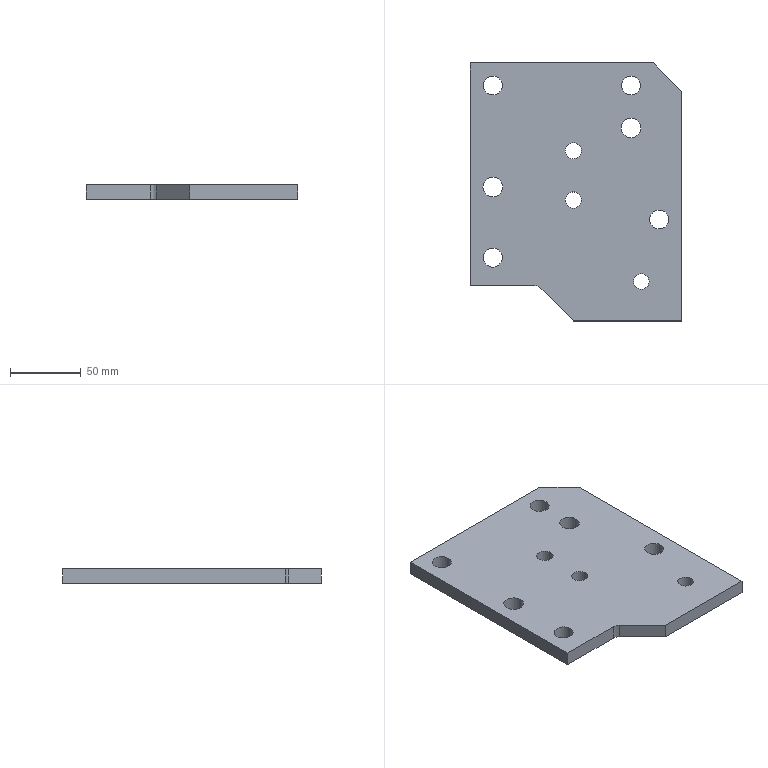Part | STEP file | lll_id126_x_t | 1 solid | 19 faces | box 150 x 183 x 10 mm | volume 245447 mm3 | cylinder 10 | plane 9 | commonest cylinder face diameters 13.509 x4 11.5 x2 14 x2 11 x1 12 x1
STEP:
#1=CARTESIAN_POINT('',(691.354,184.425,92.5));
#2=VERTEX_POINT('',#1);
#3=CARTESIAN_POINT('',(821.354,184.425,92.5));
#4=VERTEX_POINT('',#3);
#5=CARTESIAN_POINT('',(691.354,184.425,92.5));
#6=DIRECTION('',(1.,0.,0.));
#7=VECTOR('',#6,1.);
#8=LINE('',#5,#7);
#9=EDGE_CURVE('',#2,#4,#8,.T.);
#10=ORIENTED_EDGE('',*,*,#9,.T.);
#11=CARTESIAN_POINT('',(841.354,164.425,92.5));
#12=VERTEX_POINT('',#11);
#13=CARTESIAN_POINT('',(502.889,502.889,92.5));
#14=DIRECTION('',(0.7071,-0.7071,0.));
#15=VECTOR('',#14,1.);
#16=LINE('',#13,#15);
#17=EDGE_CURVE('',#4,#12,#16,.T.);
#18=ORIENTED_EDGE('',*,*,#17,.T.);
#19=CARTESIAN_POINT('',(841.354,1.425,92.5));
#20=VERTEX_POINT('',#19);
#21=CARTESIAN_POINT('',(841.354,0.,92.5));
#22=DIRECTION('',(0.,-1.,0.));
#23=VECTOR('',#22,1.);
#24=LINE('',#21,#23);
#25=EDGE_CURVE('',#12,#20,#24,.T.);
#26=ORIENTED_EDGE('',*,*,#25,.T.);
#27=CARTESIAN_POINT('',(764.739,1.425,92.5));
#28=VERTEX_POINT('',#27);
#29=CARTESIAN_POINT('',(0.,1.425,92.5));
#30=DIRECTION('',(-1.,0.,0.));
#31=VECTOR('',#30,1.);
#32=LINE('',#29,#31);
#33=EDGE_CURVE('',#20,#28,#32,.T.);
#34=ORIENTED_EDGE('',*,*,#33,.T.);
#35=CARTESIAN_POINT('',(741.497,24.668,92.5));
#36=VERTEX_POINT('',#35);
#37=CARTESIAN_POINT('',(739.739,26.425,92.5));
#38=DIRECTION('',(0.7071,-0.7071,0.));
#39=VECTOR('',#38,1.);
#40=LINE('',#37,#39);
#41=EDGE_CURVE('',#36,#28,#40,.T.);
#42=ORIENTED_EDGE('',*,*,#41,.F.);
#43=CARTESIAN_POINT('',(737.254,26.425,92.5));
#44=VERTEX_POINT('',#43);
#45=CARTESIAN_POINT('',(737.254,20.425,92.5));
#46=DIRECTION('',(0.,0.,1.));
#47=DIRECTION('',(-1.,0.,0.));
#48=AXIS2_PLACEMENT_3D('',#45,#46,#47);
#49=CIRCLE('',#48,6.);
#50=EDGE_CURVE('',#36,#44,#49,.T.);
#51=ORIENTED_EDGE('',*,*,#50,.T.);
#52=CARTESIAN_POINT('',(691.354,26.425,92.5));
#53=VERTEX_POINT('',#52);
#54=CARTESIAN_POINT('',(821.354,26.425,92.5));
#55=DIRECTION('',(-1.,0.,0.));
#56=VECTOR('',#55,1.);
#57=LINE('',#54,#56);
#58=EDGE_CURVE('',#44,#53,#57,.T.);
#59=ORIENTED_EDGE('',*,*,#58,.T.);
#60=CARTESIAN_POINT('',(691.354,26.425,92.5));
#61=DIRECTION('',(0.,1.,0.));
#62=VECTOR('',#61,1.);
#63=LINE('',#60,#62);
#64=EDGE_CURVE('',#53,#2,#63,.T.);
#65=ORIENTED_EDGE('',*,*,#64,.T.);
#66=EDGE_LOOP('',(#10,#18,#26,#34,#42,#51,#59,#65));
#67=FACE_BOUND('',#66,.T.);
#68=CARTESIAN_POINT('',(758.725,122.222,92.5));
#69=VERTEX_POINT('',#68);
#70=CARTESIAN_POINT('',(764.475,122.222,92.5));
#71=DIRECTION('',(0.,0.,-1.));
#72=DIRECTION('',(-1.,0.,0.));
#73=AXIS2_PLACEMENT_3D('',#70,#71,#72);
#74=CIRCLE('',#73,5.75);
#75=EDGE_CURVE('',#69,#69,#74,.T.);
#76=ORIENTED_EDGE('',*,*,#75,.F.);
#77=EDGE_LOOP('',(#76));
#78=FACE_BOUND('',#77,.T.);
#79=CARTESIAN_POINT('',(798.599,168.425,92.5));
#80=VERTEX_POINT('',#79);
#81=CARTESIAN_POINT('',(805.354,168.425,92.5));
#82=DIRECTION('',(0.,0.,1.));
#83=DIRECTION('',(-1.,0.,0.));
#84=AXIS2_PLACEMENT_3D('',#81,#82,#83);
#85=CIRCLE('',#84,6.755);
#86=EDGE_CURVE('',#80,#80,#85,.T.);
#87=ORIENTED_EDGE('',*,*,#86,.T.);
#88=EDGE_LOOP('',(#87));
#89=FACE_BOUND('',#88,.T.);
#90=CARTESIAN_POINT('',(700.599,168.425,92.5));
#91=VERTEX_POINT('',#90);
#92=CARTESIAN_POINT('',(707.354,168.425,92.5));
#93=DIRECTION('',(0.,0.,1.));
#94=DIRECTION('',(-1.,0.,0.));
#95=AXIS2_PLACEMENT_3D('',#92,#93,#94);
#96=CIRCLE('',#95,6.755);
#97=EDGE_CURVE('',#91,#91,#96,.T.);
#98=ORIENTED_EDGE('',*,*,#97,.T.);
#99=EDGE_LOOP('',(#98));
#100=FACE_BOUND('',#99,.T.);
#101=CARTESIAN_POINT('',(798.353,138.425,92.5));
#102=VERTEX_POINT('',#101);
#103=CARTESIAN_POINT('',(805.354,138.425,92.5));
#104=DIRECTION('',(0.,0.,1.));
#105=DIRECTION('',(-1.,0.,0.));
#106=AXIS2_PLACEMENT_3D('',#103,#104,#105);
#107=CIRCLE('',#106,7.);
#108=EDGE_CURVE('',#102,#102,#107,.T.);
#109=ORIENTED_EDGE('',*,*,#108,.T.);
#110=EDGE_LOOP('',(#109));
#111=FACE_BOUND('',#110,.T.);
#112=CARTESIAN_POINT('',(700.353,96.425,92.5));
#113=VERTEX_POINT('',#112);
#114=CARTESIAN_POINT('',(707.354,96.425,92.5));
#115=DIRECTION('',(0.,0.,1.));
#116=DIRECTION('',(-1.,0.,0.));
#117=AXIS2_PLACEMENT_3D('',#114,#115,#116);
#118=CIRCLE('',#117,7.);
#119=EDGE_CURVE('',#113,#113,#118,.T.);
#120=ORIENTED_EDGE('',*,*,#119,.T.);
#121=EDGE_LOOP('',(#120));
#122=FACE_BOUND('',#121,.T.);
#123=CARTESIAN_POINT('',(818.599,73.425,92.5));
#124=VERTEX_POINT('',#123);
#125=CARTESIAN_POINT('',(825.354,73.425,92.5));
#126=DIRECTION('',(0.,0.,1.));
#127=DIRECTION('',(-1.,0.,0.));
#128=AXIS2_PLACEMENT_3D('',#125,#126,#127);
#129=CIRCLE('',#128,6.755);
#130=EDGE_CURVE('',#124,#124,#129,.T.);
#131=ORIENTED_EDGE('',*,*,#130,.T.);
#132=EDGE_LOOP('',(#131));
#133=FACE_BOUND('',#132,.T.);
#134=CARTESIAN_POINT('',(700.599,46.425,92.5));
#135=VERTEX_POINT('',#134);
#136=CARTESIAN_POINT('',(707.354,46.425,92.5));
#137=DIRECTION('',(0.,0.,1.));
#138=DIRECTION('',(-1.,0.,0.));
#139=AXIS2_PLACEMENT_3D('',#136,#137,#138);
#140=CIRCLE('',#139,6.755);
#141=EDGE_CURVE('',#135,#135,#140,.T.);
#142=ORIENTED_EDGE('',*,*,#141,.T.);
#143=EDGE_LOOP('',(#142));
#144=FACE_BOUND('',#143,.T.);
#145=CARTESIAN_POINT('',(758.725,87.222,92.5));
#146=VERTEX_POINT('',#145);
#147=CARTESIAN_POINT('',(764.475,87.222,92.5));
#148=DIRECTION('',(0.,0.,1.));
#149=DIRECTION('',(-1.,0.,0.));
#150=AXIS2_PLACEMENT_3D('',#147,#148,#149);
#151=CIRCLE('',#150,5.75);
#152=EDGE_CURVE('',#146,#146,#151,.T.);
#153=ORIENTED_EDGE('',*,*,#152,.T.);
#154=EDGE_LOOP('',(#153));
#155=FACE_BOUND('',#154,.T.);
#156=CARTESIAN_POINT('',(807.232,29.42,92.5));
#157=VERTEX_POINT('',#156);
#158=CARTESIAN_POINT('',(812.732,29.42,92.5));
#159=DIRECTION('',(0.,0.,1.));
#160=DIRECTION('',(-1.,0.,0.));
#161=AXIS2_PLACEMENT_3D('',#158,#159,#160);
#162=CIRCLE('',#161,5.5);
#163=EDGE_CURVE('',#157,#157,#162,.T.);
#164=ORIENTED_EDGE('',*,*,#163,.T.);
#165=EDGE_LOOP('',(#164));
#166=FACE_BOUND('',#165,.T.);
#167=CARTESIAN_POINT('',(0.,0.,92.5));
#168=DIRECTION('',(0.,0.,-1.));
#169=DIRECTION('',(1.,0.,0.));
#170=AXIS2_PLACEMENT_3D('',#167,#168,#169);
#171=PLANE('',#170);
#172=ADVANCED_FACE('',(#67,#78,#89,#100,#111,#122,#133,#144,#155,#166),#171,.T.);
#173=CARTESIAN_POINT('',(807.232,29.42,102.5));
#174=VERTEX_POINT('',#173);
#175=CARTESIAN_POINT('',(812.732,29.42,102.5));
#176=DIRECTION('',(0.,0.,-1.));
#177=DIRECTION('',(-1.,0.,0.));
#178=AXIS2_PLACEMENT_3D('',#175,#176,#177);
#179=CIRCLE('',#178,5.5);
#180=EDGE_CURVE('',#174,#174,#179,.T.);
#181=ORIENTED_EDGE('',*,*,#180,.T.);
#182=EDGE_LOOP('',(#181));
#183=FACE_BOUND('',#182,.T.);
#184=CARTESIAN_POINT('',(841.354,164.425,102.5));
#185=VERTEX_POINT('',#184);
#186=CARTESIAN_POINT('',(841.354,1.425,102.5));
#187=VERTEX_POINT('',#186);
#188=CARTESIAN_POINT('',(841.354,0.,102.5));
#189=DIRECTION('',(0.,-1.,0.));
#190=VECTOR('',#189,1.);
#191=LINE('',#188,#190);
#192=EDGE_CURVE('',#185,#187,#191,.T.);
#193=ORIENTED_EDGE('',*,*,#192,.F.);
#194=CARTESIAN_POINT('',(821.354,184.425,102.5));
#195=VERTEX_POINT('',#194);
#196=CARTESIAN_POINT('',(821.354,184.425,102.5));
#197=DIRECTION('',(-0.7071,0.7071,0.));
#198=VECTOR('',#197,1.);
#199=LINE('',#196,#198);
#200=EDGE_CURVE('',#185,#195,#199,.T.);
#201=ORIENTED_EDGE('',*,*,#200,.T.);
#202=CARTESIAN_POINT('',(691.354,184.425,102.5));
#203=VERTEX_POINT('',#202);
#204=CARTESIAN_POINT('',(691.354,184.425,102.5));
#205=DIRECTION('',(1.,0.,0.));
#206=VECTOR('',#205,1.);
#207=LINE('',#204,#206);
#208=EDGE_CURVE('',#203,#195,#207,.T.);
#209=ORIENTED_EDGE('',*,*,#208,.F.);
#210=CARTESIAN_POINT('',(691.354,26.425,102.5));
#211=VERTEX_POINT('',#210);
#212=CARTESIAN_POINT('',(691.354,26.425,102.5));
#213=DIRECTION('',(0.,1.,0.));
#214=VECTOR('',#213,1.);
#215=LINE('',#212,#214);
#216=EDGE_CURVE('',#211,#203,#215,.T.);
#217=ORIENTED_EDGE('',*,*,#216,.F.);
#218=CARTESIAN_POINT('',(737.254,26.425,102.5));
#219=VERTEX_POINT('',#218);
#220=CARTESIAN_POINT('',(821.354,26.425,102.5));
#221=DIRECTION('',(-1.,0.,0.));
#222=VECTOR('',#221,1.);
#223=LINE('',#220,#222);
#224=EDGE_CURVE('',#219,#211,#223,.T.);
#225=ORIENTED_EDGE('',*,*,#224,.F.);
#226=CARTESIAN_POINT('',(741.497,24.668,102.5));
#227=VERTEX_POINT('',#226);
#228=CARTESIAN_POINT('',(737.254,20.425,102.5));
#229=DIRECTION('',(0.,0.,-1.));
#230=DIRECTION('',(-1.,0.,0.));
#231=AXIS2_PLACEMENT_3D('',#228,#229,#230);
#232=CIRCLE('',#231,6.);
#233=EDGE_CURVE('',#219,#227,#232,.T.);
#234=ORIENTED_EDGE('',*,*,#233,.T.);
#235=CARTESIAN_POINT('',(764.739,1.425,102.5));
#236=VERTEX_POINT('',#235);
#237=CARTESIAN_POINT('',(739.739,26.425,102.5));
#238=DIRECTION('',(0.7071,-0.7071,0.));
#239=VECTOR('',#238,1.);
#240=LINE('',#237,#239);
#241=EDGE_CURVE('',#227,#236,#240,.T.);
#242=ORIENTED_EDGE('',*,*,#241,.T.);
#243=CARTESIAN_POINT('',(0.,1.425,102.5));
#244=DIRECTION('',(-1.,0.,0.));
#245=VECTOR('',#244,1.);
#246=LINE('',#243,#245);
#247=EDGE_CURVE('',#187,#236,#246,.T.);
#248=ORIENTED_EDGE('',*,*,#247,.F.);
#249=EDGE_LOOP('',(#193,#201,#209,#217,#225,#234,#242,#248));
#250=FACE_BOUND('',#249,.T.);
#251=CARTESIAN_POINT('',(758.725,87.222,102.5));
#252=VERTEX_POINT('',#251);
#253=CARTESIAN_POINT('',(764.475,87.222,102.5));
#254=DIRECTION('',(0.,0.,1.));
#255=DIRECTION('',(-1.,0.,0.));
#256=AXIS2_PLACEMENT_3D('',#253,#254,#255);
#257=CIRCLE('',#256,5.75);
#258=EDGE_CURVE('',#252,#252,#257,.T.);
#259=ORIENTED_EDGE('',*,*,#258,.F.);
#260=EDGE_LOOP('',(#259));
#261=FACE_BOUND('',#260,.T.);
#262=CARTESIAN_POINT('',(700.599,46.425,102.5));
#263=VERTEX_POINT('',#262);
#264=CARTESIAN_POINT('',(707.354,46.425,102.5));
#265=DIRECTION('',(0.,0.,1.));
#266=DIRECTION('',(-1.,0.,0.));
#267=AXIS2_PLACEMENT_3D('',#264,#265,#266);
#268=CIRCLE('',#267,6.755);
#269=EDGE_CURVE('',#263,#263,#268,.T.);
#270=ORIENTED_EDGE('',*,*,#269,.F.);
#271=EDGE_LOOP('',(#270));
#272=FACE_BOUND('',#271,.T.);
#273=CARTESIAN_POINT('',(818.599,73.425,102.5));
#274=VERTEX_POINT('',#273);
#275=CARTESIAN_POINT('',(825.354,73.425,102.5));
#276=DIRECTION('',(0.,0.,1.));
#277=DIRECTION('',(-1.,0.,0.));
#278=AXIS2_PLACEMENT_3D('',#275,#276,#277);
#279=CIRCLE('',#278,6.755);
#280=EDGE_CURVE('',#274,#274,#279,.T.);
#281=ORIENTED_EDGE('',*,*,#280,.F.);
#282=EDGE_LOOP('',(#281));
#283=FACE_BOUND('',#282,.T.);
#284=CARTESIAN_POINT('',(700.353,96.425,102.5));
#285=VERTEX_POINT('',#284);
#286=CARTESIAN_POINT('',(707.354,96.425,102.5));
#287=DIRECTION('',(0.,0.,1.));
#288=DIRECTION('',(-1.,0.,0.));
#289=AXIS2_PLACEMENT_3D('',#286,#287,#288);
#290=CIRCLE('',#289,7.);
#291=EDGE_CURVE('',#285,#285,#290,.T.);
#292=ORIENTED_EDGE('',*,*,#291,.F.);
#293=EDGE_LOOP('',(#292));
#294=FACE_BOUND('',#293,.T.);
#295=CARTESIAN_POINT('',(798.353,138.425,102.5));
#296=VERTEX_POINT('',#295);
#297=CARTESIAN_POINT('',(805.354,138.425,102.5));
#298=DIRECTION('',(0.,0.,1.));
#299=DIRECTION('',(-1.,0.,0.));
#300=AXIS2_PLACEMENT_3D('',#297,#298,#299);
#301=CIRCLE('',#300,7.);
#302=EDGE_CURVE('',#296,#296,#301,.T.);
#303=ORIENTED_EDGE('',*,*,#302,.F.);
#304=EDGE_LOOP('',(#303));
#305=FACE_BOUND('',#304,.T.);
#306=CARTESIAN_POINT('',(700.599,168.425,102.5));
#307=VERTEX_POINT('',#306);
#308=CARTESIAN_POINT('',(707.354,168.425,102.5));
#309=DIRECTION('',(0.,0.,1.));
#310=DIRECTION('',(-1.,0.,0.));
#311=AXIS2_PLACEMENT_3D('',#308,#309,#310);
#312=CIRCLE('',#311,6.755);
#313=EDGE_CURVE('',#307,#307,#312,.T.);
#314=ORIENTED_EDGE('',*,*,#313,.F.);
#315=EDGE_LOOP('',(#314));
#316=FACE_BOUND('',#315,.T.);
#317=CARTESIAN_POINT('',(798.599,168.425,102.5));
#318=VERTEX_POINT('',#317);
#319=CARTESIAN_POINT('',(805.354,168.425,102.5));
#320=DIRECTION('',(0.,0.,1.));
#321=DIRECTION('',(-1.,0.,0.));
#322=AXIS2_PLACEMENT_3D('',#319,#320,#321);
#323=CIRCLE('',#322,6.755);
#324=EDGE_CURVE('',#318,#318,#323,.T.);
#325=ORIENTED_EDGE('',*,*,#324,.F.);
#326=EDGE_LOOP('',(#325));
#327=FACE_BOUND('',#326,.T.);
#328=CARTESIAN_POINT('',(758.725,122.222,102.5));
#329=VERTEX_POINT('',#328);
#330=CARTESIAN_POINT('',(764.475,122.222,102.5));
#331=DIRECTION('',(0.,0.,-1.));
#332=DIRECTION('',(-1.,0.,0.));
#333=AXIS2_PLACEMENT_3D('',#330,#331,#332);
#334=CIRCLE('',#333,5.75);
#335=EDGE_CURVE('',#329,#329,#334,.T.);
#336=ORIENTED_EDGE('',*,*,#335,.T.);
#337=EDGE_LOOP('',(#336));
#338=FACE_BOUND('',#337,.T.);
#339=CARTESIAN_POINT('',(0.,0.,102.5));
#340=DIRECTION('',(0.,0.,-1.));
#341=DIRECTION('',(1.,0.,0.));
#342=AXIS2_PLACEMENT_3D('',#339,#340,#341);
#343=PLANE('',#342);
#344=ADVANCED_FACE('',(#183,#250,#261,#272,#283,#294,#305,#316,#327,#338),#343,.F.);
#345=ORIENTED_EDGE('',*,*,#58,.F.);
#346=CARTESIAN_POINT('',(737.254,26.425,102.5));
#347=DIRECTION('',(0.,0.,1.));
#348=VECTOR('',#347,1.);
#349=LINE('',#346,#348);
#350=EDGE_CURVE('',#44,#219,#349,.T.);
#351=ORIENTED_EDGE('',*,*,#350,.T.);
#352=ORIENTED_EDGE('',*,*,#224,.T.);
#353=CARTESIAN_POINT('',(691.354,26.425,102.5));
#354=DIRECTION('',(0.,0.,-1.));
#355=VECTOR('',#354,1.);
#356=LINE('',#353,#355);
#357=EDGE_CURVE('',#211,#53,#356,.T.);
#358=ORIENTED_EDGE('',*,*,#357,.T.);
#359=EDGE_LOOP('',(#345,#351,#352,#358));
#360=FACE_OUTER_BOUND('',#359,.T.);
#361=CARTESIAN_POINT('',(821.354,26.425,102.5));
#362=DIRECTION('',(0.,-1.,0.));
#363=DIRECTION('',(0.,0.,1.));
#364=AXIS2_PLACEMENT_3D('',#361,#362,#363);
#365=PLANE('',#364);
#366=ADVANCED_FACE('',(#360),#365,.T.);
#367=ORIENTED_EDGE('',*,*,#25,.F.);
#368=CARTESIAN_POINT('',(841.354,164.425,102.5));
#369=DIRECTION('',(0.,0.,1.));
#370=VECTOR('',#369,1.);
#371=LINE('',#368,#370);
#372=EDGE_CURVE('',#12,#185,#371,.T.);
#373=ORIENTED_EDGE('',*,*,#372,.T.);
#374=ORIENTED_EDGE('',*,*,#192,.T.);
#375=CARTESIAN_POINT('',(841.354,1.425,102.5));
#376=DIRECTION('',(0.,0.,-1.));
#377=VECTOR('',#376,1.);
#378=LINE('',#375,#377);
#379=EDGE_CURVE('',#187,#20,#378,.T.);
#380=ORIENTED_EDGE('',*,*,#379,.T.);
#381=EDGE_LOOP('',(#367,#373,#374,#380));
#382=FACE_OUTER_BOUND('',#381,.T.);
#383=CARTESIAN_POINT('',(841.354,184.425,102.5));
#384=DIRECTION('',(1.,0.,0.));
#385=DIRECTION('',(0.,0.,1.));
#386=AXIS2_PLACEMENT_3D('',#383,#384,#385);
#387=PLANE('',#386);
#388=ADVANCED_FACE('',(#382),#387,.T.);
#389=ORIENTED_EDGE('',*,*,#208,.T.);
#390=CARTESIAN_POINT('',(821.354,184.425,102.5));
#391=DIRECTION('',(0.,0.,-1.));
#392=VECTOR('',#391,1.);
#393=LINE('',#390,#392);
#394=EDGE_CURVE('',#195,#4,#393,.T.);
#395=ORIENTED_EDGE('',*,*,#394,.T.);
#396=ORIENTED_EDGE('',*,*,#9,.F.);
#397=CARTESIAN_POINT('',(691.354,184.425,102.5));
#398=DIRECTION('',(0.,0.,-1.));
#399=VECTOR('',#398,1.);
#400=LINE('',#397,#399);
#401=EDGE_CURVE('',#203,#2,#400,.T.);
#402=ORIENTED_EDGE('',*,*,#401,.F.);
#403=EDGE_LOOP('',(#389,#395,#396,#402));
#404=FACE_OUTER_BOUND('',#403,.T.);
#405=CARTESIAN_POINT('',(691.354,184.425,102.5));
#406=DIRECTION('',(0.,1.,0.));
#407=DIRECTION('',(0.,0.,-1.));
#408=AXIS2_PLACEMENT_3D('',#405,#406,#407);
#409=PLANE('',#408);
#410=ADVANCED_FACE('',(#404),#409,.T.);
#411=ORIENTED_EDGE('',*,*,#313,.T.);
#412=EDGE_LOOP('',(#411));
#413=FACE_BOUND('',#412,.T.);
#414=ORIENTED_EDGE('',*,*,#97,.F.);
#415=EDGE_LOOP('',(#414));
#416=FACE_BOUND('',#415,.T.);
#417=CARTESIAN_POINT('',(707.354,168.425,102.5));
#418=DIRECTION('',(0.,0.,-1.));
#419=DIRECTION('',(1.,0.,0.));
#420=AXIS2_PLACEMENT_3D('',#417,#418,#419);
#421=CYLINDRICAL_SURFACE('',#420,6.755);
#422=ADVANCED_FACE('',(#413,#416),#421,.F.);
#423=ORIENTED_EDGE('',*,*,#302,.T.);
#424=EDGE_LOOP('',(#423));
#425=FACE_BOUND('',#424,.T.);
#426=ORIENTED_EDGE('',*,*,#108,.F.);
#427=EDGE_LOOP('',(#426));
#428=FACE_BOUND('',#427,.T.);
#429=CARTESIAN_POINT('',(805.354,138.425,102.5));
#430=DIRECTION('',(0.,0.,-1.));
#431=DIRECTION('',(1.,0.,0.));
#432=AXIS2_PLACEMENT_3D('',#429,#430,#431);
#433=CYLINDRICAL_SURFACE('',#432,7.);
#434=ADVANCED_FACE('',(#425,#428),#433,.F.);
#435=ORIENTED_EDGE('',*,*,#64,.F.);
#436=ORIENTED_EDGE('',*,*,#357,.F.);
#437=ORIENTED_EDGE('',*,*,#216,.T.);
#438=ORIENTED_EDGE('',*,*,#401,.T.);
#439=EDGE_LOOP('',(#435,#436,#437,#438));
#440=FACE_OUTER_BOUND('',#439,.T.);
#441=CARTESIAN_POINT('',(691.354,26.425,102.5));
#442=DIRECTION('',(-1.,0.,0.));
#443=DIRECTION('',(0.,0.,-1.));
#444=AXIS2_PLACEMENT_3D('',#441,#442,#443);
#445=PLANE('',#444);
#446=ADVANCED_FACE('',(#440),#445,.T.);
#447=ORIENTED_EDGE('',*,*,#291,.T.);
#448=EDGE_LOOP('',(#447));
#449=FACE_BOUND('',#448,.T.);
#450=ORIENTED_EDGE('',*,*,#119,.F.);
#451=EDGE_LOOP('',(#450));
#452=FACE_BOUND('',#451,.T.);
#453=CARTESIAN_POINT('',(707.354,96.425,102.5));
#454=DIRECTION('',(0.,0.,-1.));
#455=DIRECTION('',(1.,0.,0.));
#456=AXIS2_PLACEMENT_3D('',#453,#454,#455);
#457=CYLINDRICAL_SURFACE('',#456,7.);
#458=ADVANCED_FACE('',(#449,#452),#457,.F.);
#459=ORIENTED_EDGE('',*,*,#280,.T.);
#460=EDGE_LOOP('',(#459));
#461=FACE_BOUND('',#460,.T.);
#462=ORIENTED_EDGE('',*,*,#130,.F.);
#463=EDGE_LOOP('',(#462));
#464=FACE_BOUND('',#463,.T.);
#465=CARTESIAN_POINT('',(825.354,73.425,102.5));
#466=DIRECTION('',(0.,0.,-1.));
#467=DIRECTION('',(1.,0.,0.));
#468=AXIS2_PLACEMENT_3D('',#465,#466,#467);
#469=CYLINDRICAL_SURFACE('',#468,6.755);
#470=ADVANCED_FACE('',(#461,#464),#469,.F.);
#471=ORIENTED_EDGE('',*,*,#269,.T.);
#472=EDGE_LOOP('',(#471));
#473=FACE_BOUND('',#472,.T.);
#474=ORIENTED_EDGE('',*,*,#141,.F.);
#475=EDGE_LOOP('',(#474));
#476=FACE_BOUND('',#475,.T.);
#477=CARTESIAN_POINT('',(707.354,46.425,102.5));
#478=DIRECTION('',(0.,0.,-1.));
#479=DIRECTION('',(1.,0.,0.));
#480=AXIS2_PLACEMENT_3D('',#477,#478,#479);
#481=CYLINDRICAL_SURFACE('',#480,6.755);
#482=ADVANCED_FACE('',(#473,#476),#481,.F.);
#483=ORIENTED_EDGE('',*,*,#324,.T.);
#484=EDGE_LOOP('',(#483));
#485=FACE_BOUND('',#484,.T.);
#486=ORIENTED_EDGE('',*,*,#86,.F.);
#487=EDGE_LOOP('',(#486));
#488=FACE_BOUND('',#487,.T.);
#489=CARTESIAN_POINT('',(805.354,168.425,102.5));
#490=DIRECTION('',(0.,0.,-1.));
#491=DIRECTION('',(1.,0.,0.));
#492=AXIS2_PLACEMENT_3D('',#489,#490,#491);
#493=CYLINDRICAL_SURFACE('',#492,6.755);
#494=ADVANCED_FACE('',(#485,#488),#493,.F.);
#495=ORIENTED_EDGE('',*,*,#152,.F.);
#496=EDGE_LOOP('',(#495));
#497=FACE_BOUND('',#496,.T.);
#498=ORIENTED_EDGE('',*,*,#258,.T.);
#499=EDGE_LOOP('',(#498));
#500=FACE_BOUND('',#499,.T.);
#501=CARTESIAN_POINT('',(764.475,87.222,267.5));
#502=DIRECTION('',(0.,0.,-1.));
#503=DIRECTION('',(1.,0.,0.));
#504=AXIS2_PLACEMENT_3D('',#501,#502,#503);
#505=CYLINDRICAL_SURFACE('',#504,5.75);
#506=ADVANCED_FACE('',(#497,#500),#505,.F.);
#507=ORIENTED_EDGE('',*,*,#75,.T.);
#508=EDGE_LOOP('',(#507));
#509=FACE_BOUND('',#508,.T.);
#510=ORIENTED_EDGE('',*,*,#335,.F.);
#511=EDGE_LOOP('',(#510));
#512=FACE_BOUND('',#511,.T.);
#513=CARTESIAN_POINT('',(764.475,122.222,267.5));
#514=DIRECTION('',(0.,0.,-1.));
#515=DIRECTION('',(1.,0.,0.));
#516=AXIS2_PLACEMENT_3D('',#513,#514,#515);
#517=CYLINDRICAL_SURFACE('',#516,5.75);
#518=ADVANCED_FACE('',(#509,#512),#517,.F.);
#519=ORIENTED_EDGE('',*,*,#241,.F.);
#520=CARTESIAN_POINT('',(741.497,24.668,102.5));
#521=DIRECTION('',(0.,0.,-1.));
#522=VECTOR('',#521,1.);
#523=LINE('',#520,#522);
#524=EDGE_CURVE('',#227,#36,#523,.T.);
#525=ORIENTED_EDGE('',*,*,#524,.T.);
#526=ORIENTED_EDGE('',*,*,#41,.T.);
#527=CARTESIAN_POINT('',(764.739,1.425,102.5));
#528=DIRECTION('',(0.,0.,-1.));
#529=VECTOR('',#528,1.);
#530=LINE('',#527,#529);
#531=EDGE_CURVE('',#236,#28,#530,.T.);
#532=ORIENTED_EDGE('',*,*,#531,.F.);
#533=EDGE_LOOP('',(#519,#525,#526,#532));
#534=FACE_OUTER_BOUND('',#533,.T.);
#535=CARTESIAN_POINT('',(739.739,26.425,102.5));
#536=DIRECTION('',(0.7071,0.7071,0.));
#537=DIRECTION('',(-0.7071,0.7071,0.));
#538=AXIS2_PLACEMENT_3D('',#535,#536,#537);
#539=PLANE('',#538);
#540=ADVANCED_FACE('',(#534),#539,.F.);
#541=ORIENTED_EDGE('',*,*,#33,.F.);
#542=ORIENTED_EDGE('',*,*,#379,.F.);
#543=ORIENTED_EDGE('',*,*,#247,.T.);
#544=ORIENTED_EDGE('',*,*,#531,.T.);
#545=EDGE_LOOP('',(#541,#542,#543,#544));
#546=FACE_OUTER_BOUND('',#545,.T.);
#547=CARTESIAN_POINT('',(841.354,1.425,102.5));
#548=DIRECTION('',(0.,-1.,0.));
#549=DIRECTION('',(0.,0.,-1.));
#550=AXIS2_PLACEMENT_3D('',#547,#548,#549);
#551=PLANE('',#550);
#552=ADVANCED_FACE('',(#546),#551,.T.);
#553=ORIENTED_EDGE('',*,*,#233,.F.);
#554=ORIENTED_EDGE('',*,*,#350,.F.);
#555=ORIENTED_EDGE('',*,*,#50,.F.);
#556=ORIENTED_EDGE('',*,*,#524,.F.);
#557=EDGE_LOOP('',(#553,#554,#555,#556));
#558=FACE_OUTER_BOUND('',#557,.T.);
#559=CARTESIAN_POINT('',(737.254,20.425,102.5));
#560=DIRECTION('',(0.,0.,-1.));
#561=DIRECTION('',(-1.,0.,0.));
#562=AXIS2_PLACEMENT_3D('',#559,#560,#561);
#563=CYLINDRICAL_SURFACE('',#562,6.);
#564=ADVANCED_FACE('',(#558),#563,.F.);
#565=ORIENTED_EDGE('',*,*,#163,.F.);
#566=EDGE_LOOP('',(#565));
#567=FACE_BOUND('',#566,.T.);
#568=ORIENTED_EDGE('',*,*,#180,.F.);
#569=EDGE_LOOP('',(#568));
#570=FACE_BOUND('',#569,.T.);
#571=CARTESIAN_POINT('',(812.732,29.42,92.5));
#572=DIRECTION('',(0.,0.,1.));
#573=DIRECTION('',(1.,0.,0.));
#574=AXIS2_PLACEMENT_3D('',#571,#572,#573);
#575=CYLINDRICAL_SURFACE('',#574,5.5);
#576=ADVANCED_FACE('',(#567,#570),#575,.F.);
#577=ORIENTED_EDGE('',*,*,#200,.F.);
#578=ORIENTED_EDGE('',*,*,#372,.F.);
#579=ORIENTED_EDGE('',*,*,#17,.F.);
#580=ORIENTED_EDGE('',*,*,#394,.F.);
#581=EDGE_LOOP('',(#577,#578,#579,#580));
#582=FACE_OUTER_BOUND('',#581,.T.);
#583=CARTESIAN_POINT('',(821.354,184.425,102.5));
#584=DIRECTION('',(-0.7071,-0.7071,0.));
#585=DIRECTION('',(0.,0.,-1.));
#586=AXIS2_PLACEMENT_3D('',#583,#584,#585);
#587=PLANE('',#586);
#588=ADVANCED_FACE('',(#582),#587,.F.);
#589=CLOSED_SHELL('',(#172,#344,#366,#388,#410,#422,#434,#446,#458,#470,#482,#494,#506,#518,#540,#552,#564,#576,#588));
#590=MANIFOLD_SOLID_BREP('',#589);
#591=(LENGTH_UNIT()NAMED_UNIT(*)SI_UNIT(.MILLI.,.METRE.));
#592=UNCERTAINTY_MEASURE_WITH_UNIT(LENGTH_MEASURE(0.00002),#591,'','');
#593=(NAMED_UNIT(*)PLANE_ANGLE_UNIT()SI_UNIT($,.RADIAN.));
#594=PLANE_ANGLE_MEASURE_WITH_UNIT(PLANE_ANGLE_MEASURE(0.01745),#593);
#595=DIMENSIONAL_EXPONENTS(0.,0.,0.,0.,0.,0.,0.);
#596=(CONVERSION_BASED_UNIT('DEGREE',#594)NAMED_UNIT(#595)PLANE_ANGLE_UNIT());
#597=(NAMED_UNIT(*)SI_UNIT($,.STERADIAN.)SOLID_ANGLE_UNIT());
#598=(GEOMETRIC_REPRESENTATION_CONTEXT(3)GLOBAL_UNCERTAINTY_ASSIGNED_CONTEXT((#592))GLOBAL_UNIT_ASSIGNED_CONTEXT((#591,#596,#597))REPRESENTATION_CONTEXT('',''));
#599=ADVANCED_BREP_SHAPE_REPRESENTATION('',(#590),#598);